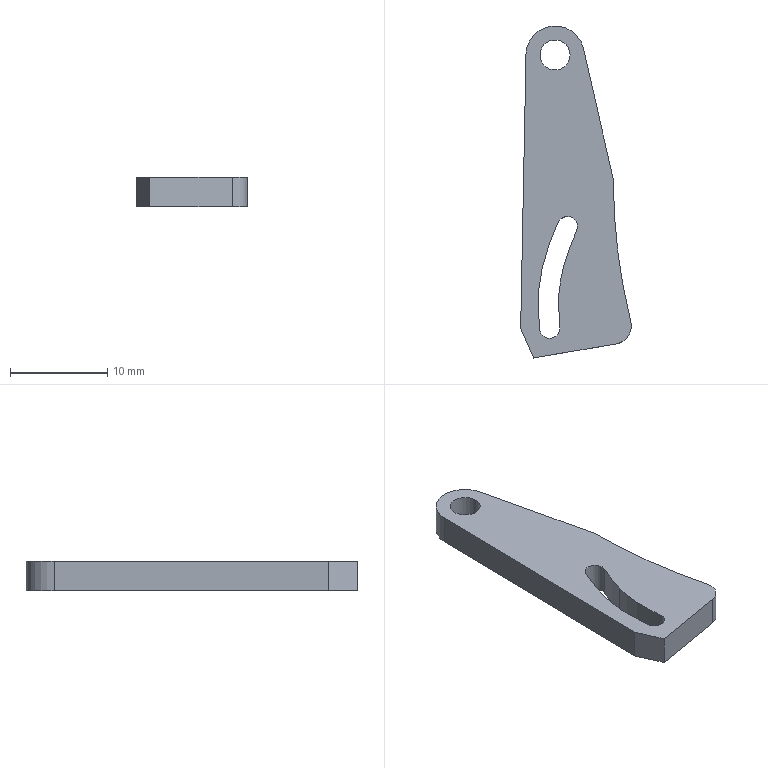Part | SolidWorks | features Extrusion 1 | 1 solid | 16 faces | box 11.407 x 34.229 x 3 mm | volume 770.437 mm3 | cylinder 7 | plane 6 | spline 3 | commonest cylinder face diameters 2.1 x2 3.1 x2 3.716 x1 6 x1 121.384 x1
STEP:
#1=CARTESIAN_POINT('',(-3.734,13.524,3.));
#2=VERTEX_POINT('',#1);
#3=CARTESIAN_POINT('',(-0.6338,13.524,3.));
#4=VERTEX_POINT('',#3);
#5=CARTESIAN_POINT('',(-2.184,13.524,3.));
#6=DIRECTION('',(0.,0.,1.));
#7=DIRECTION('',(1.,0.,0.));
#8=AXIS2_PLACEMENT_3D('',#5,#6,#7);
#9=CIRCLE('',#8,1.55);
#10=EDGE_CURVE('',#2,#4,#9,.T.);
#11=ORIENTED_EDGE('',*,*,#10,.T.);
#12=CARTESIAN_POINT('',(-0.6338,13.524,0.));
#13=VERTEX_POINT('',#12);
#14=CARTESIAN_POINT('',(-0.6338,13.524,3.));
#15=DIRECTION('',(0.,0.,-1.));
#16=VECTOR('',#15,1000.);
#17=LINE('',#14,#16);
#18=EDGE_CURVE('',#4,#13,#17,.T.);
#19=ORIENTED_EDGE('',*,*,#18,.T.);
#20=CARTESIAN_POINT('',(-3.734,13.524,0.));
#21=VERTEX_POINT('',#20);
#22=CARTESIAN_POINT('',(-2.184,13.524,0.));
#23=DIRECTION('',(0.,0.,1.));
#24=DIRECTION('',(1.,0.,0.));
#25=AXIS2_PLACEMENT_3D('',#22,#23,#24);
#26=CIRCLE('',#25,1.55);
#27=EDGE_CURVE('',#21,#13,#26,.T.);
#28=ORIENTED_EDGE('',*,*,#27,.F.);
#29=CARTESIAN_POINT('',(-3.734,13.524,3.));
#30=DIRECTION('',(0.,0.,-1.));
#31=VECTOR('',#30,1000.);
#32=LINE('',#29,#31);
#33=EDGE_CURVE('',#2,#21,#32,.T.);
#34=ORIENTED_EDGE('',*,*,#33,.F.);
#35=EDGE_LOOP('',(#11,#19,#28,#34));
#36=FACE_OUTER_BOUND('',#35,.T.);
#37=CARTESIAN_POINT('',(-2.184,13.524,3.));
#38=DIRECTION('',(0.,0.,-1.));
#39=DIRECTION('',(-1.,0.,0.));
#40=AXIS2_PLACEMENT_3D('',#37,#38,#39);
#41=CYLINDRICAL_SURFACE('',#40,1.55);
#42=ADVANCED_FACE('',(#36),#41,.F.);
#43=CARTESIAN_POINT('',(5.619,-13.971,3.));
#44=VERTEX_POINT('',#43);
#45=CARTESIAN_POINT('',(3.816,0.7114,3.));
#46=VERTEX_POINT('',#45);
#47=CARTESIAN_POINT('',(64.508,0.7114,3.));
#48=DIRECTION('',(0.,0.,-1.));
#49=DIRECTION('',(1.,0.,0.));
#50=AXIS2_PLACEMENT_3D('',#47,#48,#49);
#51=CIRCLE('',#50,60.692);
#52=EDGE_CURVE('',#44,#46,#51,.T.);
#53=ORIENTED_EDGE('',*,*,#52,.T.);
#54=CARTESIAN_POINT('',(0.7411,14.191,3.));
#55=VERTEX_POINT('',#54);
#56=CARTESIAN_POINT('',(3.816,0.7114,3.));
#57=DIRECTION('',(-0.2224,0.975,0.));
#58=VECTOR('',#57,1000.);
#59=LINE('',#56,#58);
#60=EDGE_CURVE('',#46,#55,#59,.T.);
#61=ORIENTED_EDGE('',*,*,#60,.T.);
#62=CARTESIAN_POINT('',(-5.183,13.582,3.));
#63=VERTEX_POINT('',#62);
#64=CARTESIAN_POINT('',(-2.184,13.524,3.));
#65=DIRECTION('',(0.,0.,1.));
#66=DIRECTION('',(1.,0.,0.));
#67=AXIS2_PLACEMENT_3D('',#64,#65,#66);
#68=CIRCLE('',#67,3.);
#69=EDGE_CURVE('',#55,#63,#68,.T.);
#70=ORIENTED_EDGE('',*,*,#69,.T.);
#71=CARTESIAN_POINT('',(-5.733,-14.706,3.));
#72=VERTEX_POINT('',#71);
#73=CARTESIAN_POINT('',(-5.733,-14.706,3.));
#74=DIRECTION('',(-0.01942,-0.9998,0.));
#75=VECTOR('',#74,1000.);
#76=LINE('',#73,#75);
#77=EDGE_CURVE('',#63,#72,#76,.T.);
#78=ORIENTED_EDGE('',*,*,#77,.T.);
#79=CARTESIAN_POINT('',(-4.408,-17.705,3.));
#80=VERTEX_POINT('',#79);
#81=CARTESIAN_POINT('',(-5.733,-14.706,3.));
#82=DIRECTION('',(0.404,-0.9147,0.));
#83=VECTOR('',#82,1000.);
#84=LINE('',#81,#83);
#85=EDGE_CURVE('',#72,#80,#84,.T.);
#86=ORIENTED_EDGE('',*,*,#85,.T.);
#87=CARTESIAN_POINT('',(4.128,-16.253,3.));
#88=VERTEX_POINT('',#87);
#89=CARTESIAN_POINT('',(-4.408,-17.705,3.));
#90=DIRECTION('',(0.9858,0.1677,0.));
#91=VECTOR('',#90,1000.);
#92=LINE('',#89,#91);
#93=EDGE_CURVE('',#80,#88,#92,.T.);
#94=ORIENTED_EDGE('',*,*,#93,.T.);
#95=CARTESIAN_POINT('',(3.816,-14.421,3.));
#96=DIRECTION('',(0.,0.,1.));
#97=DIRECTION('',(1.,0.,0.));
#98=AXIS2_PLACEMENT_3D('',#95,#96,#97);
#99=CIRCLE('',#98,1.858);
#100=EDGE_CURVE('',#88,#44,#99,.T.);
#101=ORIENTED_EDGE('',*,*,#100,.T.);
#102=EDGE_LOOP('',(#53,#61,#70,#78,#86,#94,#101));
#103=FACE_OUTER_BOUND('',#102,.T.);
#104=ORIENTED_EDGE('',*,*,#10,.F.);
#105=CARTESIAN_POINT('',(-2.184,13.524,3.));
#106=DIRECTION('',(0.,0.,1.));
#107=DIRECTION('',(1.,0.,0.));
#108=AXIS2_PLACEMENT_3D('',#105,#106,#107);
#109=CIRCLE('',#108,1.55);
#110=EDGE_CURVE('',#4,#2,#109,.T.);
#111=ORIENTED_EDGE('',*,*,#110,.F.);
#112=EDGE_LOOP('',(#104,#111));
#113=FACE_BOUND('',#112,.T.);
#114=CARTESIAN_POINT('',(0.03014,-4.613,3.));
#115=VERTEX_POINT('',#114);
#116=CARTESIAN_POINT('',(-1.882,-3.746,3.));
#117=VERTEX_POINT('',#116);
#118=CARTESIAN_POINT('',(-0.9217,-4.17,3.));
#119=DIRECTION('',(0.,0.,1.));
#120=DIRECTION('',(1.,0.,0.));
#121=AXIS2_PLACEMENT_3D('',#118,#119,#120);
#122=CIRCLE('',#121,1.05);
#123=EDGE_CURVE('',#115,#117,#122,.T.);
#124=ORIENTED_EDGE('',*,*,#123,.F.);
#125=CARTESIAN_POINT('',(-1.249,-8.057,3.));
#126=VERTEX_POINT('',#125);
#127=CARTESIAN_POINT('',(-1.249,-8.057,3.));
#128=CARTESIAN_POINT('',(-1.143,-7.677,3.));
#129=CARTESIAN_POINT('',(-0.9647,-7.106,3.));
#130=CARTESIAN_POINT('',(-0.6925,-6.347,3.));
#131=CARTESIAN_POINT('',(-0.3915,-5.573,3.));
#132=CARTESIAN_POINT('',(-0.1433,-4.996,3.));
#133=CARTESIAN_POINT('',(0.03014,-4.613,3.));
#134=B_SPLINE_CURVE_WITH_KNOTS('',3,(#127,#128,#129,#130,#131,#132,#133),.UNSPECIFIED.,.F.,.F.,(4,1,1,1,4),(0.,0.3221,0.4879,0.657,1.),.UNSPECIFIED.);
#135=EDGE_CURVE('',#126,#115,#134,.T.);
#136=ORIENTED_EDGE('',*,*,#135,.F.);
#137=CARTESIAN_POINT('',(-1.684,-14.605,3.));
#138=VERTEX_POINT('',#137);
#139=CARTESIAN_POINT('',(-1.684,-14.605,3.));
#140=CARTESIAN_POINT('',(-1.698,-14.231,3.));
#141=CARTESIAN_POINT('',(-1.691,-13.651,3.));
#142=CARTESIAN_POINT('',(-1.791,-12.908,3.));
#143=CARTESIAN_POINT('',(-1.82,-12.364,3.));
#144=CARTESIAN_POINT('',(-1.823,-11.845,3.));
#145=CARTESIAN_POINT('',(-1.807,-11.32,3.));
#146=CARTESIAN_POINT('',(-1.768,-10.788,3.));
#147=CARTESIAN_POINT('',(-1.708,-10.252,3.));
#148=CARTESIAN_POINT('',(-1.625,-9.71,3.));
#149=CARTESIAN_POINT('',(-1.486,-8.974,3.));
#150=CARTESIAN_POINT('',(-1.351,-8.424,3.));
#151=CARTESIAN_POINT('',(-1.249,-8.057,3.));
#152=B_SPLINE_CURVE_WITH_KNOTS('',3,(#139,#140,#141,#142,#143,#144,#145,#146,#147,#148,#149,#150,#151),.UNSPECIFIED.,.F.,.F.,(4,1,1,1,1,1,1,1,1,1,4),(0.,0.1704,0.2623,0.34,0.4178,0.4978,0.5783,0.66,0.7429,0.8271,1.),.UNSPECIFIED.);
#153=EDGE_CURVE('',#138,#126,#152,.T.);
#154=ORIENTED_EDGE('',*,*,#153,.F.);
#155=CARTESIAN_POINT('',(-3.783,-14.657,3.));
#156=VERTEX_POINT('',#155);
#157=CARTESIAN_POINT('',(-2.734,-14.631,3.));
#158=DIRECTION('',(0.,0.,1.));
#159=DIRECTION('',(1.,0.,0.));
#160=AXIS2_PLACEMENT_3D('',#157,#158,#159);
#161=CIRCLE('',#160,1.05);
#162=EDGE_CURVE('',#156,#138,#161,.T.);
#163=ORIENTED_EDGE('',*,*,#162,.F.);
#164=CARTESIAN_POINT('',(-1.882,-3.746,3.));
#165=CARTESIAN_POINT('',(-2.072,-4.165,3.));
#166=CARTESIAN_POINT('',(-2.343,-4.794,3.));
#167=CARTESIAN_POINT('',(-2.67,-5.641,3.));
#168=CARTESIAN_POINT('',(-2.896,-6.271,3.));
#169=CARTESIAN_POINT('',(-3.101,-6.899,3.));
#170=CARTESIAN_POINT('',(-3.284,-7.526,3.));
#171=CARTESIAN_POINT('',(-3.447,-8.152,3.));
#172=CARTESIAN_POINT('',(-3.586,-8.776,3.));
#173=CARTESIAN_POINT('',(-3.741,-9.604,3.));
#174=CARTESIAN_POINT('',(-3.849,-10.432,3.));
#175=CARTESIAN_POINT('',(-3.907,-11.258,3.));
#176=CARTESIAN_POINT('',(-3.924,-11.873,3.));
#177=CARTESIAN_POINT('',(-3.916,-12.486,3.));
#178=CARTESIAN_POINT('',(-3.886,-13.056,3.));
#179=CARTESIAN_POINT('',(-3.786,-13.774,3.));
#180=CARTESIAN_POINT('',(-3.799,-14.298,3.));
#181=CARTESIAN_POINT('',(-3.783,-14.657,3.));
#182=B_SPLINE_CURVE_WITH_KNOTS('',3,(#164,#165,#166,#167,#168,#169,#170,#171,#172,#173,#174,#175,#176,#177,#178,#179,#180,#181),.UNSPECIFIED.,.F.,.F.,(4,1,1,1,1,1,1,1,1,1,1,1,1,1,1,4),(0.,0.1228,0.183,0.2425,0.3014,0.3595,0.4171,0.4741,0.5305,0.6419,0.697,0.7515,0.8064,0.8607,0.9038,1.),.UNSPECIFIED.);
#183=EDGE_CURVE('',#117,#156,#182,.T.);
#184=ORIENTED_EDGE('',*,*,#183,.F.);
#185=EDGE_LOOP('',(#124,#136,#154,#163,#184));
#186=FACE_BOUND('',#185,.T.);
#187=CARTESIAN_POINT('',(64.508,0.7114,3.));
#188=DIRECTION('',(0.,0.,1.));
#189=DIRECTION('',(1.,0.,0.));
#190=AXIS2_PLACEMENT_3D('',#187,#188,#189);
#191=PLANE('',#190);
#192=ADVANCED_FACE('',(#103,#113,#186),#191,.T.);
#193=ORIENTED_EDGE('',*,*,#27,.T.);
#194=CARTESIAN_POINT('',(-2.184,13.524,0.));
#195=DIRECTION('',(0.,0.,1.));
#196=DIRECTION('',(1.,0.,0.));
#197=AXIS2_PLACEMENT_3D('',#194,#195,#196);
#198=CIRCLE('',#197,1.55);
#199=EDGE_CURVE('',#13,#21,#198,.T.);
#200=ORIENTED_EDGE('',*,*,#199,.T.);
#201=EDGE_LOOP('',(#193,#200));
#202=FACE_BOUND('',#201,.T.);
#203=CARTESIAN_POINT('',(5.619,-13.971,0.));
#204=VERTEX_POINT('',#203);
#205=CARTESIAN_POINT('',(3.816,0.7114,0.));
#206=VERTEX_POINT('',#205);
#207=CARTESIAN_POINT('',(64.508,0.7114,0.));
#208=DIRECTION('',(0.,0.,-1.));
#209=DIRECTION('',(1.,0.,0.));
#210=AXIS2_PLACEMENT_3D('',#207,#208,#209);
#211=CIRCLE('',#210,60.692);
#212=EDGE_CURVE('',#204,#206,#211,.T.);
#213=ORIENTED_EDGE('',*,*,#212,.F.);
#214=CARTESIAN_POINT('',(4.128,-16.253,0.));
#215=VERTEX_POINT('',#214);
#216=CARTESIAN_POINT('',(3.816,-14.421,0.));
#217=DIRECTION('',(0.,0.,1.));
#218=DIRECTION('',(1.,0.,0.));
#219=AXIS2_PLACEMENT_3D('',#216,#217,#218);
#220=CIRCLE('',#219,1.858);
#221=EDGE_CURVE('',#215,#204,#220,.T.);
#222=ORIENTED_EDGE('',*,*,#221,.F.);
#223=CARTESIAN_POINT('',(-4.408,-17.705,0.));
#224=VERTEX_POINT('',#223);
#225=CARTESIAN_POINT('',(-4.408,-17.705,0.));
#226=DIRECTION('',(0.9858,0.1677,0.));
#227=VECTOR('',#226,1000.);
#228=LINE('',#225,#227);
#229=EDGE_CURVE('',#224,#215,#228,.T.);
#230=ORIENTED_EDGE('',*,*,#229,.F.);
#231=CARTESIAN_POINT('',(-5.733,-14.706,0.));
#232=VERTEX_POINT('',#231);
#233=CARTESIAN_POINT('',(-5.733,-14.706,0.));
#234=DIRECTION('',(0.404,-0.9147,0.));
#235=VECTOR('',#234,1000.);
#236=LINE('',#233,#235);
#237=EDGE_CURVE('',#232,#224,#236,.T.);
#238=ORIENTED_EDGE('',*,*,#237,.F.);
#239=CARTESIAN_POINT('',(-5.183,13.582,0.));
#240=VERTEX_POINT('',#239);
#241=CARTESIAN_POINT('',(-5.733,-14.706,0.));
#242=DIRECTION('',(-0.01942,-0.9998,0.));
#243=VECTOR('',#242,1000.);
#244=LINE('',#241,#243);
#245=EDGE_CURVE('',#240,#232,#244,.T.);
#246=ORIENTED_EDGE('',*,*,#245,.F.);
#247=CARTESIAN_POINT('',(0.7411,14.191,0.));
#248=VERTEX_POINT('',#247);
#249=CARTESIAN_POINT('',(-2.184,13.524,0.));
#250=DIRECTION('',(0.,0.,1.));
#251=DIRECTION('',(1.,0.,0.));
#252=AXIS2_PLACEMENT_3D('',#249,#250,#251);
#253=CIRCLE('',#252,3.);
#254=EDGE_CURVE('',#248,#240,#253,.T.);
#255=ORIENTED_EDGE('',*,*,#254,.F.);
#256=CARTESIAN_POINT('',(3.816,0.7114,0.));
#257=DIRECTION('',(-0.2224,0.975,0.));
#258=VECTOR('',#257,1000.);
#259=LINE('',#256,#258);
#260=EDGE_CURVE('',#206,#248,#259,.T.);
#261=ORIENTED_EDGE('',*,*,#260,.F.);
#262=EDGE_LOOP('',(#213,#222,#230,#238,#246,#255,#261));
#263=FACE_OUTER_BOUND('',#262,.T.);
#264=CARTESIAN_POINT('',(-1.249,-8.057,0.));
#265=VERTEX_POINT('',#264);
#266=CARTESIAN_POINT('',(0.03014,-4.613,0.));
#267=VERTEX_POINT('',#266);
#268=CARTESIAN_POINT('',(-1.249,-8.057,0.));
#269=CARTESIAN_POINT('',(-1.143,-7.677,0.));
#270=CARTESIAN_POINT('',(-0.9647,-7.106,0.));
#271=CARTESIAN_POINT('',(-0.6925,-6.347,0.));
#272=CARTESIAN_POINT('',(-0.3915,-5.573,0.));
#273=CARTESIAN_POINT('',(-0.1433,-4.996,0.));
#274=CARTESIAN_POINT('',(0.03014,-4.613,0.));
#275=B_SPLINE_CURVE_WITH_KNOTS('',3,(#268,#269,#270,#271,#272,#273,#274),.UNSPECIFIED.,.F.,.F.,(4,1,1,1,4),(0.,0.3221,0.4879,0.657,1.),.UNSPECIFIED.);
#276=EDGE_CURVE('',#265,#267,#275,.T.);
#277=ORIENTED_EDGE('',*,*,#276,.T.);
#278=CARTESIAN_POINT('',(-1.882,-3.746,0.));
#279=VERTEX_POINT('',#278);
#280=CARTESIAN_POINT('',(-0.9217,-4.17,0.));
#281=DIRECTION('',(0.,0.,1.));
#282=DIRECTION('',(1.,0.,0.));
#283=AXIS2_PLACEMENT_3D('',#280,#281,#282);
#284=CIRCLE('',#283,1.05);
#285=EDGE_CURVE('',#267,#279,#284,.T.);
#286=ORIENTED_EDGE('',*,*,#285,.T.);
#287=CARTESIAN_POINT('',(-3.783,-14.657,0.));
#288=VERTEX_POINT('',#287);
#289=CARTESIAN_POINT('',(-1.882,-3.746,0.));
#290=CARTESIAN_POINT('',(-2.072,-4.165,0.));
#291=CARTESIAN_POINT('',(-2.343,-4.794,0.));
#292=CARTESIAN_POINT('',(-2.67,-5.641,0.));
#293=CARTESIAN_POINT('',(-2.896,-6.271,0.));
#294=CARTESIAN_POINT('',(-3.101,-6.899,0.));
#295=CARTESIAN_POINT('',(-3.284,-7.526,0.));
#296=CARTESIAN_POINT('',(-3.447,-8.152,0.));
#297=CARTESIAN_POINT('',(-3.586,-8.776,0.));
#298=CARTESIAN_POINT('',(-3.741,-9.604,0.));
#299=CARTESIAN_POINT('',(-3.849,-10.432,0.));
#300=CARTESIAN_POINT('',(-3.907,-11.258,0.));
#301=CARTESIAN_POINT('',(-3.924,-11.873,0.));
#302=CARTESIAN_POINT('',(-3.916,-12.486,0.));
#303=CARTESIAN_POINT('',(-3.886,-13.056,0.));
#304=CARTESIAN_POINT('',(-3.786,-13.774,0.));
#305=CARTESIAN_POINT('',(-3.799,-14.298,0.));
#306=CARTESIAN_POINT('',(-3.783,-14.657,0.));
#307=B_SPLINE_CURVE_WITH_KNOTS('',3,(#289,#290,#291,#292,#293,#294,#295,#296,#297,#298,#299,#300,#301,#302,#303,#304,#305,#306),.UNSPECIFIED.,.F.,.F.,(4,1,1,1,1,1,1,1,1,1,1,1,1,1,1,4),(0.,0.1228,0.183,0.2425,0.3014,0.3595,0.4171,0.4741,0.5305,0.6419,0.697,0.7515,0.8064,0.8607,0.9038,1.),.UNSPECIFIED.);
#308=EDGE_CURVE('',#279,#288,#307,.T.);
#309=ORIENTED_EDGE('',*,*,#308,.T.);
#310=CARTESIAN_POINT('',(-1.684,-14.605,0.));
#311=VERTEX_POINT('',#310);
#312=CARTESIAN_POINT('',(-2.734,-14.631,0.));
#313=DIRECTION('',(0.,0.,1.));
#314=DIRECTION('',(1.,0.,0.));
#315=AXIS2_PLACEMENT_3D('',#312,#313,#314);
#316=CIRCLE('',#315,1.05);
#317=EDGE_CURVE('',#288,#311,#316,.T.);
#318=ORIENTED_EDGE('',*,*,#317,.T.);
#319=CARTESIAN_POINT('',(-1.684,-14.605,0.));
#320=CARTESIAN_POINT('',(-1.698,-14.231,0.));
#321=CARTESIAN_POINT('',(-1.691,-13.651,0.));
#322=CARTESIAN_POINT('',(-1.791,-12.908,0.));
#323=CARTESIAN_POINT('',(-1.82,-12.364,0.));
#324=CARTESIAN_POINT('',(-1.823,-11.845,0.));
#325=CARTESIAN_POINT('',(-1.807,-11.32,0.));
#326=CARTESIAN_POINT('',(-1.768,-10.788,0.));
#327=CARTESIAN_POINT('',(-1.708,-10.252,0.));
#328=CARTESIAN_POINT('',(-1.625,-9.71,0.));
#329=CARTESIAN_POINT('',(-1.486,-8.974,0.));
#330=CARTESIAN_POINT('',(-1.351,-8.424,0.));
#331=CARTESIAN_POINT('',(-1.249,-8.057,0.));
#332=B_SPLINE_CURVE_WITH_KNOTS('',3,(#319,#320,#321,#322,#323,#324,#325,#326,#327,#328,#329,#330,#331),.UNSPECIFIED.,.F.,.F.,(4,1,1,1,1,1,1,1,1,1,4),(0.,0.1704,0.2623,0.34,0.4178,0.4978,0.5783,0.66,0.7429,0.8271,1.),.UNSPECIFIED.);
#333=EDGE_CURVE('',#311,#265,#332,.T.);
#334=ORIENTED_EDGE('',*,*,#333,.T.);
#335=EDGE_LOOP('',(#277,#286,#309,#318,#334));
#336=FACE_BOUND('',#335,.T.);
#337=CARTESIAN_POINT('',(64.508,0.7114,0.));
#338=DIRECTION('',(0.,0.,1.));
#339=DIRECTION('',(1.,0.,0.));
#340=AXIS2_PLACEMENT_3D('',#337,#338,#339);
#341=PLANE('',#340);
#342=ADVANCED_FACE('',(#202,#263,#336),#341,.F.);
#343=ORIENTED_EDGE('',*,*,#212,.T.);
#344=CARTESIAN_POINT('',(3.816,0.7114,3.));
#345=DIRECTION('',(0.,0.,-1.));
#346=VECTOR('',#345,1000.);
#347=LINE('',#344,#346);
#348=EDGE_CURVE('',#46,#206,#347,.T.);
#349=ORIENTED_EDGE('',*,*,#348,.F.);
#350=ORIENTED_EDGE('',*,*,#52,.F.);
#351=CARTESIAN_POINT('',(5.619,-13.971,3.));
#352=DIRECTION('',(0.,0.,-1.));
#353=VECTOR('',#352,1000.);
#354=LINE('',#351,#353);
#355=EDGE_CURVE('',#44,#204,#354,.T.);
#356=ORIENTED_EDGE('',*,*,#355,.T.);
#357=EDGE_LOOP('',(#343,#349,#350,#356));
#358=FACE_OUTER_BOUND('',#357,.T.);
#359=CARTESIAN_POINT('',(64.508,0.7114,3.));
#360=DIRECTION('',(0.,0.,-1.));
#361=DIRECTION('',(-1.,0.,0.));
#362=AXIS2_PLACEMENT_3D('',#359,#360,#361);
#363=CYLINDRICAL_SURFACE('',#362,60.692);
#364=ADVANCED_FACE('',(#358),#363,.F.);
#365=ORIENTED_EDGE('',*,*,#260,.T.);
#366=CARTESIAN_POINT('',(0.7411,14.191,3.));
#367=DIRECTION('',(0.,0.,-1.));
#368=VECTOR('',#367,1000.);
#369=LINE('',#366,#368);
#370=EDGE_CURVE('',#55,#248,#369,.T.);
#371=ORIENTED_EDGE('',*,*,#370,.F.);
#372=ORIENTED_EDGE('',*,*,#60,.F.);
#373=ORIENTED_EDGE('',*,*,#348,.T.);
#374=EDGE_LOOP('',(#365,#371,#372,#373));
#375=FACE_OUTER_BOUND('',#374,.T.);
#376=CARTESIAN_POINT('',(3.816,0.7114,3.));
#377=DIRECTION('',(-0.975,-0.2224,0.));
#378=DIRECTION('',(0.2224,-0.975,0.));
#379=AXIS2_PLACEMENT_3D('',#376,#377,#378);
#380=PLANE('',#379);
#381=ADVANCED_FACE('',(#375),#380,.F.);
#382=ORIENTED_EDGE('',*,*,#254,.T.);
#383=CARTESIAN_POINT('',(-5.183,13.582,3.));
#384=DIRECTION('',(0.,0.,-1.));
#385=VECTOR('',#384,1000.);
#386=LINE('',#383,#385);
#387=EDGE_CURVE('',#63,#240,#386,.T.);
#388=ORIENTED_EDGE('',*,*,#387,.F.);
#389=ORIENTED_EDGE('',*,*,#69,.F.);
#390=ORIENTED_EDGE('',*,*,#370,.T.);
#391=EDGE_LOOP('',(#382,#388,#389,#390));
#392=FACE_OUTER_BOUND('',#391,.T.);
#393=CARTESIAN_POINT('',(-2.184,13.524,3.));
#394=DIRECTION('',(0.,0.,-1.));
#395=DIRECTION('',(-1.,0.,0.));
#396=AXIS2_PLACEMENT_3D('',#393,#394,#395);
#397=CYLINDRICAL_SURFACE('',#396,3.);
#398=ADVANCED_FACE('',(#392),#397,.T.);
#399=ORIENTED_EDGE('',*,*,#245,.T.);
#400=CARTESIAN_POINT('',(-5.733,-14.706,3.));
#401=DIRECTION('',(0.,0.,-1.));
#402=VECTOR('',#401,1000.);
#403=LINE('',#400,#402);
#404=EDGE_CURVE('',#72,#232,#403,.T.);
#405=ORIENTED_EDGE('',*,*,#404,.F.);
#406=ORIENTED_EDGE('',*,*,#77,.F.);
#407=ORIENTED_EDGE('',*,*,#387,.T.);
#408=EDGE_LOOP('',(#399,#405,#406,#407));
#409=FACE_OUTER_BOUND('',#408,.T.);
#410=CARTESIAN_POINT('',(-5.733,-14.706,3.));
#411=DIRECTION('',(0.9998,-0.01942,0.));
#412=DIRECTION('',(0.01942,0.9998,0.));
#413=AXIS2_PLACEMENT_3D('',#410,#411,#412);
#414=PLANE('',#413);
#415=ADVANCED_FACE('',(#409),#414,.F.);
#416=ORIENTED_EDGE('',*,*,#237,.T.);
#417=CARTESIAN_POINT('',(-4.408,-17.705,3.));
#418=DIRECTION('',(0.,0.,-1.));
#419=VECTOR('',#418,1000.);
#420=LINE('',#417,#419);
#421=EDGE_CURVE('',#80,#224,#420,.T.);
#422=ORIENTED_EDGE('',*,*,#421,.F.);
#423=ORIENTED_EDGE('',*,*,#85,.F.);
#424=ORIENTED_EDGE('',*,*,#404,.T.);
#425=EDGE_LOOP('',(#416,#422,#423,#424));
#426=FACE_OUTER_BOUND('',#425,.T.);
#427=CARTESIAN_POINT('',(-5.733,-14.706,3.));
#428=DIRECTION('',(0.9147,0.404,0.));
#429=DIRECTION('',(-0.404,0.9147,0.));
#430=AXIS2_PLACEMENT_3D('',#427,#428,#429);
#431=PLANE('',#430);
#432=ADVANCED_FACE('',(#426),#431,.F.);
#433=ORIENTED_EDGE('',*,*,#229,.T.);
#434=CARTESIAN_POINT('',(4.128,-16.253,3.));
#435=DIRECTION('',(0.,0.,-1.));
#436=VECTOR('',#435,1000.);
#437=LINE('',#434,#436);
#438=EDGE_CURVE('',#88,#215,#437,.T.);
#439=ORIENTED_EDGE('',*,*,#438,.F.);
#440=ORIENTED_EDGE('',*,*,#93,.F.);
#441=ORIENTED_EDGE('',*,*,#421,.T.);
#442=EDGE_LOOP('',(#433,#439,#440,#441));
#443=FACE_OUTER_BOUND('',#442,.T.);
#444=CARTESIAN_POINT('',(-4.408,-17.705,3.));
#445=DIRECTION('',(-0.1677,0.9858,0.));
#446=DIRECTION('',(-0.9858,-0.1677,0.));
#447=AXIS2_PLACEMENT_3D('',#444,#445,#446);
#448=PLANE('',#447);
#449=ADVANCED_FACE('',(#443),#448,.F.);
#450=ORIENTED_EDGE('',*,*,#221,.T.);
#451=ORIENTED_EDGE('',*,*,#355,.F.);
#452=ORIENTED_EDGE('',*,*,#100,.F.);
#453=ORIENTED_EDGE('',*,*,#438,.T.);
#454=EDGE_LOOP('',(#450,#451,#452,#453));
#455=FACE_OUTER_BOUND('',#454,.T.);
#456=CARTESIAN_POINT('',(3.816,-14.421,3.));
#457=DIRECTION('',(0.,0.,-1.));
#458=DIRECTION('',(-1.,0.,0.));
#459=AXIS2_PLACEMENT_3D('',#456,#457,#458);
#460=CYLINDRICAL_SURFACE('',#459,1.858);
#461=ADVANCED_FACE('',(#455),#460,.T.);
#462=ORIENTED_EDGE('',*,*,#18,.F.);
#463=ORIENTED_EDGE('',*,*,#110,.T.);
#464=ORIENTED_EDGE('',*,*,#33,.T.);
#465=ORIENTED_EDGE('',*,*,#199,.F.);
#466=EDGE_LOOP('',(#462,#463,#464,#465));
#467=FACE_OUTER_BOUND('',#466,.T.);
#468=CARTESIAN_POINT('',(-2.184,13.524,3.));
#469=DIRECTION('',(0.,0.,-1.));
#470=DIRECTION('',(-1.,0.,0.));
#471=AXIS2_PLACEMENT_3D('',#468,#469,#470);
#472=CYLINDRICAL_SURFACE('',#471,1.55);
#473=ADVANCED_FACE('',(#467),#472,.F.);
#474=ORIENTED_EDGE('',*,*,#276,.F.);
#475=CARTESIAN_POINT('',(-1.249,-8.057,3.));
#476=DIRECTION('',(0.,0.,-1.));
#477=VECTOR('',#476,1000.);
#478=LINE('',#475,#477);
#479=EDGE_CURVE('',#126,#265,#478,.T.);
#480=ORIENTED_EDGE('',*,*,#479,.F.);
#481=ORIENTED_EDGE('',*,*,#135,.T.);
#482=CARTESIAN_POINT('',(0.03014,-4.613,3.));
#483=DIRECTION('',(0.,0.,-1.));
#484=VECTOR('',#483,1000.);
#485=LINE('',#482,#484);
#486=EDGE_CURVE('',#115,#267,#485,.T.);
#487=ORIENTED_EDGE('',*,*,#486,.T.);
#488=EDGE_LOOP('',(#474,#480,#481,#487));
#489=FACE_OUTER_BOUND('',#488,.T.);
#490=CARTESIAN_POINT('',(-1.249,-8.057,3.));
#491=CARTESIAN_POINT('',(-1.249,-8.057,0.));
#492=CARTESIAN_POINT('',(-1.143,-7.677,3.));
#493=CARTESIAN_POINT('',(-1.143,-7.677,0.));
#494=CARTESIAN_POINT('',(-0.9647,-7.106,3.));
#495=CARTESIAN_POINT('',(-0.9647,-7.106,0.));
#496=CARTESIAN_POINT('',(-0.6925,-6.347,3.));
#497=CARTESIAN_POINT('',(-0.6925,-6.347,0.));
#498=CARTESIAN_POINT('',(-0.3915,-5.573,3.));
#499=CARTESIAN_POINT('',(-0.3915,-5.573,0.));
#500=CARTESIAN_POINT('',(-0.1433,-4.996,3.));
#501=CARTESIAN_POINT('',(-0.1433,-4.996,0.));
#502=CARTESIAN_POINT('',(0.03014,-4.613,3.));
#503=CARTESIAN_POINT('',(0.03014,-4.613,0.));
#504=B_SPLINE_SURFACE_WITH_KNOTS('',3,1,((#490,#491),(#492,#493),(#494,#495),(#496,#497),(#498,#499),(#500,#501),(#502,#503)),.UNSPECIFIED.,.F.,.F.,.F.,(4,1,1,1,4),(2,2),(0.,0.3221,0.4879,0.657,1.),(0.,1.),.UNSPECIFIED.);
#505=ADVANCED_FACE('',(#489),#504,.T.);
#506=ORIENTED_EDGE('',*,*,#285,.F.);
#507=ORIENTED_EDGE('',*,*,#486,.F.);
#508=ORIENTED_EDGE('',*,*,#123,.T.);
#509=CARTESIAN_POINT('',(-1.882,-3.746,3.));
#510=DIRECTION('',(0.,0.,-1.));
#511=VECTOR('',#510,1000.);
#512=LINE('',#509,#511);
#513=EDGE_CURVE('',#117,#279,#512,.T.);
#514=ORIENTED_EDGE('',*,*,#513,.T.);
#515=EDGE_LOOP('',(#506,#507,#508,#514));
#516=FACE_OUTER_BOUND('',#515,.T.);
#517=CARTESIAN_POINT('',(-0.9217,-4.17,3.));
#518=DIRECTION('',(0.,0.,-1.));
#519=DIRECTION('',(-1.,0.,0.));
#520=AXIS2_PLACEMENT_3D('',#517,#518,#519);
#521=CYLINDRICAL_SURFACE('',#520,1.05);
#522=ADVANCED_FACE('',(#516),#521,.F.);
#523=ORIENTED_EDGE('',*,*,#308,.F.);
#524=ORIENTED_EDGE('',*,*,#513,.F.);
#525=ORIENTED_EDGE('',*,*,#183,.T.);
#526=CARTESIAN_POINT('',(-3.783,-14.657,3.));
#527=DIRECTION('',(0.,0.,-1.));
#528=VECTOR('',#527,1000.);
#529=LINE('',#526,#528);
#530=EDGE_CURVE('',#156,#288,#529,.T.);
#531=ORIENTED_EDGE('',*,*,#530,.T.);
#532=EDGE_LOOP('',(#523,#524,#525,#531));
#533=FACE_OUTER_BOUND('',#532,.T.);
#534=CARTESIAN_POINT('',(-1.882,-3.746,3.));
#535=CARTESIAN_POINT('',(-1.882,-3.746,0.));
#536=CARTESIAN_POINT('',(-2.072,-4.165,3.));
#537=CARTESIAN_POINT('',(-2.072,-4.165,0.));
#538=CARTESIAN_POINT('',(-2.343,-4.794,3.));
#539=CARTESIAN_POINT('',(-2.343,-4.794,0.));
#540=CARTESIAN_POINT('',(-2.67,-5.641,3.));
#541=CARTESIAN_POINT('',(-2.67,-5.641,0.));
#542=CARTESIAN_POINT('',(-2.896,-6.271,3.));
#543=CARTESIAN_POINT('',(-2.896,-6.271,0.));
#544=CARTESIAN_POINT('',(-3.101,-6.899,3.));
#545=CARTESIAN_POINT('',(-3.101,-6.899,0.));
#546=CARTESIAN_POINT('',(-3.284,-7.526,3.));
#547=CARTESIAN_POINT('',(-3.284,-7.526,0.));
#548=CARTESIAN_POINT('',(-3.447,-8.152,3.));
#549=CARTESIAN_POINT('',(-3.447,-8.152,0.));
#550=CARTESIAN_POINT('',(-3.586,-8.776,3.));
#551=CARTESIAN_POINT('',(-3.586,-8.776,0.));
#552=CARTESIAN_POINT('',(-3.741,-9.604,3.));
#553=CARTESIAN_POINT('',(-3.741,-9.604,0.));
#554=CARTESIAN_POINT('',(-3.849,-10.432,3.));
#555=CARTESIAN_POINT('',(-3.849,-10.432,0.));
#556=CARTESIAN_POINT('',(-3.907,-11.258,3.));
#557=CARTESIAN_POINT('',(-3.907,-11.258,0.));
#558=CARTESIAN_POINT('',(-3.924,-11.873,3.));
#559=CARTESIAN_POINT('',(-3.924,-11.873,0.));
#560=CARTESIAN_POINT('',(-3.916,-12.486,3.));
#561=CARTESIAN_POINT('',(-3.916,-12.486,0.));
#562=CARTESIAN_POINT('',(-3.886,-13.056,3.));
#563=CARTESIAN_POINT('',(-3.886,-13.056,0.));
#564=CARTESIAN_POINT('',(-3.786,-13.774,3.));
#565=CARTESIAN_POINT('',(-3.786,-13.774,0.));
#566=CARTESIAN_POINT('',(-3.799,-14.298,3.));
#567=CARTESIAN_POINT('',(-3.799,-14.298,0.));
#568=CARTESIAN_POINT('',(-3.783,-14.657,3.));
#569=CARTESIAN_POINT('',(-3.783,-14.657,0.));
#570=B_SPLINE_SURFACE_WITH_KNOTS('',3,1,((#534,#535),(#536,#537),(#538,#539),(#540,#541),(#542,#543),(#544,#545),(#546,#547),(#548,#549),(#550,#551),(#552,#553),(#554,#555),(#556,#557),(#558,#559),(#560,#561),(#562,#563),(#564,#565),(#566,#567),(#568,#569)),.UNSPECIFIED.,.F.,.F.,.F.,(4,1,1,1,1,1,1,1,1,1,1,1,1,1,1,4),(2,2),(0.,0.1228,0.183,0.2425,0.3014,0.3595,0.4171,0.4741,0.5305,0.6419,0.697,0.7515,0.8064,0.8607,0.9038,1.),(0.,1.),.UNSPECIFIED.);
#571=ADVANCED_FACE('',(#533),#570,.T.);
#572=ORIENTED_EDGE('',*,*,#317,.F.);
#573=ORIENTED_EDGE('',*,*,#530,.F.);
#574=ORIENTED_EDGE('',*,*,#162,.T.);
#575=CARTESIAN_POINT('',(-1.684,-14.605,3.));
#576=DIRECTION('',(0.,0.,-1.));
#577=VECTOR('',#576,1000.);
#578=LINE('',#575,#577);
#579=EDGE_CURVE('',#138,#311,#578,.T.);
#580=ORIENTED_EDGE('',*,*,#579,.T.);
#581=EDGE_LOOP('',(#572,#573,#574,#580));
#582=FACE_OUTER_BOUND('',#581,.T.);
#583=CARTESIAN_POINT('',(-2.734,-14.631,3.));
#584=DIRECTION('',(0.,0.,-1.));
#585=DIRECTION('',(-1.,0.,0.));
#586=AXIS2_PLACEMENT_3D('',#583,#584,#585);
#587=CYLINDRICAL_SURFACE('',#586,1.05);
#588=ADVANCED_FACE('',(#582),#587,.F.);
#589=ORIENTED_EDGE('',*,*,#333,.F.);
#590=ORIENTED_EDGE('',*,*,#579,.F.);
#591=ORIENTED_EDGE('',*,*,#153,.T.);
#592=ORIENTED_EDGE('',*,*,#479,.T.);
#593=EDGE_LOOP('',(#589,#590,#591,#592));
#594=FACE_OUTER_BOUND('',#593,.T.);
#595=CARTESIAN_POINT('',(-1.684,-14.605,3.));
#596=CARTESIAN_POINT('',(-1.684,-14.605,0.));
#597=CARTESIAN_POINT('',(-1.698,-14.231,3.));
#598=CARTESIAN_POINT('',(-1.698,-14.231,0.));
#599=CARTESIAN_POINT('',(-1.691,-13.651,3.));
#600=CARTESIAN_POINT('',(-1.691,-13.651,0.));
#601=CARTESIAN_POINT('',(-1.791,-12.908,3.));
#602=CARTESIAN_POINT('',(-1.791,-12.908,0.));
#603=CARTESIAN_POINT('',(-1.82,-12.364,3.));
#604=CARTESIAN_POINT('',(-1.82,-12.364,0.));
#605=CARTESIAN_POINT('',(-1.823,-11.845,3.));
#606=CARTESIAN_POINT('',(-1.823,-11.845,0.));
#607=CARTESIAN_POINT('',(-1.807,-11.32,3.));
#608=CARTESIAN_POINT('',(-1.807,-11.32,0.));
#609=CARTESIAN_POINT('',(-1.768,-10.788,3.));
#610=CARTESIAN_POINT('',(-1.768,-10.788,0.));
#611=CARTESIAN_POINT('',(-1.708,-10.252,3.));
#612=CARTESIAN_POINT('',(-1.708,-10.252,0.));
#613=CARTESIAN_POINT('',(-1.625,-9.71,3.));
#614=CARTESIAN_POINT('',(-1.625,-9.71,0.));
#615=CARTESIAN_POINT('',(-1.486,-8.974,3.));
#616=CARTESIAN_POINT('',(-1.486,-8.974,0.));
#617=CARTESIAN_POINT('',(-1.351,-8.424,3.));
#618=CARTESIAN_POINT('',(-1.351,-8.424,0.));
#619=CARTESIAN_POINT('',(-1.249,-8.057,3.));
#620=CARTESIAN_POINT('',(-1.249,-8.057,0.));
#621=B_SPLINE_SURFACE_WITH_KNOTS('',3,1,((#595,#596),(#597,#598),(#599,#600),(#601,#602),(#603,#604),(#605,#606),(#607,#608),(#609,#610),(#611,#612),(#613,#614),(#615,#616),(#617,#618),(#619,#620)),.UNSPECIFIED.,.F.,.F.,.F.,(4,1,1,1,1,1,1,1,1,1,4),(2,2),(0.,0.1704,0.2623,0.34,0.4178,0.4978,0.5783,0.66,0.7429,0.8271,1.),(0.,1.),.UNSPECIFIED.);
#622=ADVANCED_FACE('',(#594),#621,.T.);
#623=CLOSED_SHELL('',(#42,#192,#342,#364,#381,#398,#415,#432,#449,#461,#473,#505,#522,#571,#588,#622));
#624=MANIFOLD_SOLID_BREP('',#623);
#625=CARTESIAN_POINT('',(0.,0.,0.));
#626=DIRECTION('',(0.,0.,1.));
#627=DIRECTION('',(1.,0.,0.));
#628=AXIS2_PLACEMENT_3D('',#625,#626,#627);
#629=(LENGTH_UNIT()NAMED_UNIT(*)SI_UNIT(.MILLI.,.METRE.));
#630=UNCERTAINTY_MEASURE_WITH_UNIT(LENGTH_MEASURE(0.00001),#629,'','');
#631=(NAMED_UNIT(*)PLANE_ANGLE_UNIT()SI_UNIT($,.RADIAN.));
#632=(NAMED_UNIT(*)SI_UNIT($,.STERADIAN.)SOLID_ANGLE_UNIT());
#633=(GEOMETRIC_REPRESENTATION_CONTEXT(3)GLOBAL_UNCERTAINTY_ASSIGNED_CONTEXT((#630))GLOBAL_UNIT_ASSIGNED_CONTEXT((#629,#631,#632))REPRESENTATION_CONTEXT('',''));
#634=ADVANCED_BREP_SHAPE_REPRESENTATION('',(#624,#628),#633);